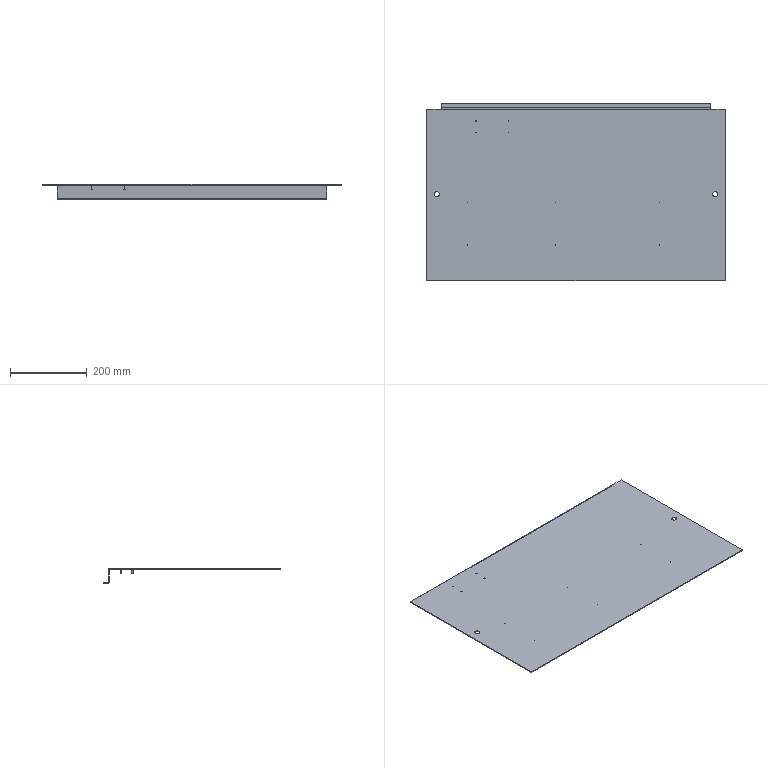Part | NX | features solid 2 | 1 solid | 64 faces | box 776 x 461.5 x 40 mm | volume 763535 mm3 | cylinder 38 | plane 26 | commonest cylinder face diameters 1 x20 4 x10 13 x4 6 x2 8 x2